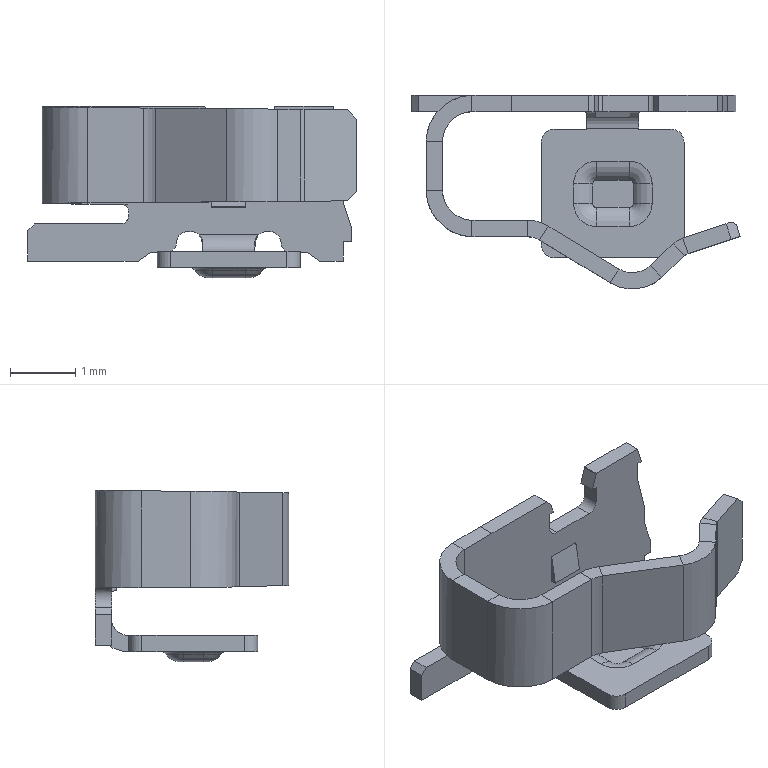Part | NX | 1 solid | 141 faces | box 5.018 x 2.959 x 2.622 mm | volume 5.774 mm3 | plane 89 | cylinder 38 | torus 12 | spline 2 | commonest cylinder face diameters 0.3 x6 0.2 x5 0.5 x5 0.7 x5 0.35 x4 0.4 x4